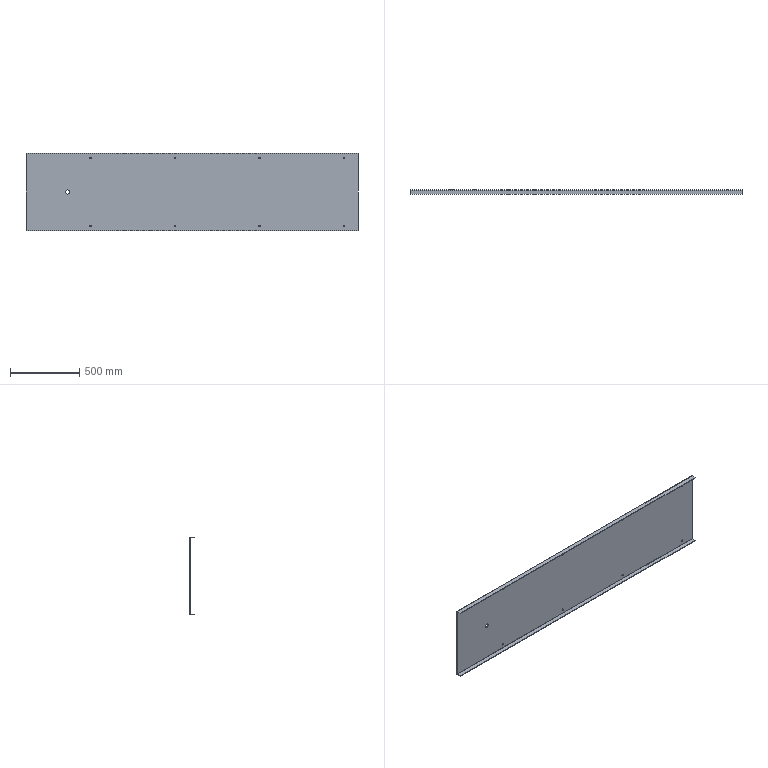Part | STEP file | Input 116 | 1 solid | 32 faces | box 2395 x 35 x 559 mm | volume 6649356 mm3 | cylinder 22 | plane 10 | commonest cylinder face diameters 12 x16 1 x2 10 x2 30 x2